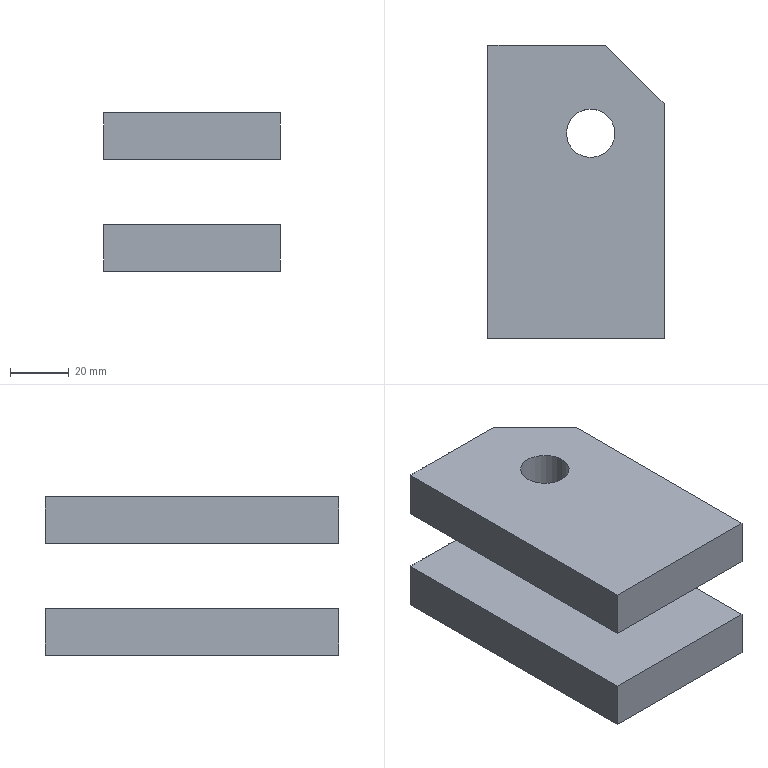Part | SolidWorks | features Chamfer 1, Extrusion 1, ICE 1, MirrorSolid 1 | 2 solids | 18 faces | box 60 x 100 x 54 mm | volume 178758 mm3 | plane 14 | cylinder 4 | commonest cylinder face diameters 16.5 x4
STEP:
#1=CARTESIAN_POINT('',(-3.25,20.,0.));
#2=VERTEX_POINT('',#1);
#3=CARTESIAN_POINT('',(13.25,20.,0.));
#4=VERTEX_POINT('',#3);
#5=CARTESIAN_POINT('',(5.,20.,0.));
#6=DIRECTION('',(0.,0.,1.));
#7=DIRECTION('',(1.,0.,0.));
#8=AXIS2_PLACEMENT_3D('',#5,#6,#7);
#9=CIRCLE('',#8,8.25);
#10=EDGE_CURVE('',#2,#4,#9,.T.);
#11=ORIENTED_EDGE('',*,*,#10,.F.);
#12=CARTESIAN_POINT('',(-3.25,20.,16.));
#13=VERTEX_POINT('',#12);
#14=CARTESIAN_POINT('',(-3.25,20.,0.));
#15=DIRECTION('',(0.,0.,1.));
#16=VECTOR('',#15,1000.);
#17=LINE('',#14,#16);
#18=EDGE_CURVE('',#2,#13,#17,.T.);
#19=ORIENTED_EDGE('',*,*,#18,.T.);
#20=CARTESIAN_POINT('',(13.25,20.,16.));
#21=VERTEX_POINT('',#20);
#22=CARTESIAN_POINT('',(5.,20.,16.));
#23=DIRECTION('',(0.,0.,1.));
#24=DIRECTION('',(1.,0.,0.));
#25=AXIS2_PLACEMENT_3D('',#22,#23,#24);
#26=CIRCLE('',#25,8.25);
#27=EDGE_CURVE('',#13,#21,#26,.T.);
#28=ORIENTED_EDGE('',*,*,#27,.T.);
#29=CARTESIAN_POINT('',(13.25,20.,0.));
#30=DIRECTION('',(0.,0.,1.));
#31=VECTOR('',#30,1000.);
#32=LINE('',#29,#31);
#33=EDGE_CURVE('',#4,#21,#32,.T.);
#34=ORIENTED_EDGE('',*,*,#33,.F.);
#35=EDGE_LOOP('',(#11,#19,#28,#34));
#36=FACE_OUTER_BOUND('',#35,.T.);
#37=CARTESIAN_POINT('',(5.,20.,0.));
#38=DIRECTION('',(0.,0.,1.));
#39=DIRECTION('',(1.,0.,0.));
#40=AXIS2_PLACEMENT_3D('',#37,#38,#39);
#41=CYLINDRICAL_SURFACE('',#40,8.25);
#42=ADVANCED_FACE('',(#36),#41,.F.);
#43=CARTESIAN_POINT('',(30.,-50.,0.));
#44=VERTEX_POINT('',#43);
#45=CARTESIAN_POINT('',(30.,30.,0.));
#46=VERTEX_POINT('',#45);
#47=CARTESIAN_POINT('',(30.,-50.,0.));
#48=DIRECTION('',(0.,1.,0.));
#49=VECTOR('',#48,1000.);
#50=LINE('',#47,#49);
#51=EDGE_CURVE('',#44,#46,#50,.T.);
#52=ORIENTED_EDGE('',*,*,#51,.T.);
#53=CARTESIAN_POINT('',(30.,30.,16.));
#54=VERTEX_POINT('',#53);
#55=CARTESIAN_POINT('',(30.,30.,16.));
#56=DIRECTION('',(0.,0.,1.));
#57=VECTOR('',#56,1000.);
#58=LINE('',#55,#57);
#59=EDGE_CURVE('',#46,#54,#58,.T.);
#60=ORIENTED_EDGE('',*,*,#59,.T.);
#61=CARTESIAN_POINT('',(30.,-50.,16.));
#62=VERTEX_POINT('',#61);
#63=CARTESIAN_POINT('',(30.,-50.,16.));
#64=DIRECTION('',(0.,1.,0.));
#65=VECTOR('',#64,1000.);
#66=LINE('',#63,#65);
#67=EDGE_CURVE('',#62,#54,#66,.T.);
#68=ORIENTED_EDGE('',*,*,#67,.F.);
#69=CARTESIAN_POINT('',(30.,-50.,16.));
#70=DIRECTION('',(0.,0.,-1.));
#71=VECTOR('',#70,1000.);
#72=LINE('',#69,#71);
#73=EDGE_CURVE('',#62,#44,#72,.T.);
#74=ORIENTED_EDGE('',*,*,#73,.T.);
#75=EDGE_LOOP('',(#52,#60,#68,#74));
#76=FACE_OUTER_BOUND('',#75,.T.);
#77=CARTESIAN_POINT('',(30.,-50.,16.));
#78=DIRECTION('',(-1.,0.,0.));
#79=DIRECTION('',(0.,0.,1.));
#80=AXIS2_PLACEMENT_3D('',#77,#78,#79);
#81=PLANE('',#80);
#82=ADVANCED_FACE('',(#76),#81,.F.);
#83=CARTESIAN_POINT('',(10.,50.,16.));
#84=VERTEX_POINT('',#83);
#85=CARTESIAN_POINT('',(-30.,50.,16.));
#86=VERTEX_POINT('',#85);
#87=CARTESIAN_POINT('',(-30.,50.,16.));
#88=DIRECTION('',(-1.,0.,0.));
#89=VECTOR('',#88,1000.);
#90=LINE('',#87,#89);
#91=EDGE_CURVE('',#84,#86,#90,.T.);
#92=ORIENTED_EDGE('',*,*,#91,.F.);
#93=CARTESIAN_POINT('',(10.,50.,0.));
#94=VERTEX_POINT('',#93);
#95=CARTESIAN_POINT('',(10.,50.,16.));
#96=DIRECTION('',(0.,0.,-1.));
#97=VECTOR('',#96,1000.);
#98=LINE('',#95,#97);
#99=EDGE_CURVE('',#84,#94,#98,.T.);
#100=ORIENTED_EDGE('',*,*,#99,.T.);
#101=CARTESIAN_POINT('',(-30.,50.,0.));
#102=VERTEX_POINT('',#101);
#103=CARTESIAN_POINT('',(-30.,50.,0.));
#104=DIRECTION('',(-1.,0.,0.));
#105=VECTOR('',#104,1000.);
#106=LINE('',#103,#105);
#107=EDGE_CURVE('',#94,#102,#106,.T.);
#108=ORIENTED_EDGE('',*,*,#107,.T.);
#109=CARTESIAN_POINT('',(-30.,50.,16.));
#110=DIRECTION('',(0.,0.,-1.));
#111=VECTOR('',#110,1000.);
#112=LINE('',#109,#111);
#113=EDGE_CURVE('',#86,#102,#112,.T.);
#114=ORIENTED_EDGE('',*,*,#113,.F.);
#115=EDGE_LOOP('',(#92,#100,#108,#114));
#116=FACE_OUTER_BOUND('',#115,.T.);
#117=CARTESIAN_POINT('',(-30.,50.,16.));
#118=DIRECTION('',(0.,-1.,0.));
#119=DIRECTION('',(0.,0.,-1.));
#120=AXIS2_PLACEMENT_3D('',#117,#118,#119);
#121=PLANE('',#120);
#122=ADVANCED_FACE('',(#116),#121,.F.);
#123=CARTESIAN_POINT('',(-30.,-50.,0.));
#124=VERTEX_POINT('',#123);
#125=CARTESIAN_POINT('',(-30.,-50.,0.));
#126=DIRECTION('',(0.,-1.,0.));
#127=VECTOR('',#126,1000.);
#128=LINE('',#125,#127);
#129=EDGE_CURVE('',#102,#124,#128,.T.);
#130=ORIENTED_EDGE('',*,*,#129,.T.);
#131=CARTESIAN_POINT('',(-30.,-50.,16.));
#132=VERTEX_POINT('',#131);
#133=CARTESIAN_POINT('',(-30.,-50.,16.));
#134=DIRECTION('',(0.,0.,-1.));
#135=VECTOR('',#134,1000.);
#136=LINE('',#133,#135);
#137=EDGE_CURVE('',#132,#124,#136,.T.);
#138=ORIENTED_EDGE('',*,*,#137,.F.);
#139=CARTESIAN_POINT('',(-30.,-50.,16.));
#140=DIRECTION('',(0.,-1.,0.));
#141=VECTOR('',#140,1000.);
#142=LINE('',#139,#141);
#143=EDGE_CURVE('',#86,#132,#142,.T.);
#144=ORIENTED_EDGE('',*,*,#143,.F.);
#145=ORIENTED_EDGE('',*,*,#113,.T.);
#146=EDGE_LOOP('',(#130,#138,#144,#145));
#147=FACE_OUTER_BOUND('',#146,.T.);
#148=CARTESIAN_POINT('',(-30.,-50.,16.));
#149=DIRECTION('',(1.,0.,0.));
#150=DIRECTION('',(0.,0.,-1.));
#151=AXIS2_PLACEMENT_3D('',#148,#149,#150);
#152=PLANE('',#151);
#153=ADVANCED_FACE('',(#147),#152,.F.);
#154=CARTESIAN_POINT('',(-30.,-50.,0.));
#155=DIRECTION('',(1.,0.,0.));
#156=VECTOR('',#155,1000.);
#157=LINE('',#154,#156);
#158=EDGE_CURVE('',#124,#44,#157,.T.);
#159=ORIENTED_EDGE('',*,*,#158,.T.);
#160=ORIENTED_EDGE('',*,*,#73,.F.);
#161=CARTESIAN_POINT('',(-30.,-50.,16.));
#162=DIRECTION('',(1.,0.,0.));
#163=VECTOR('',#162,1000.);
#164=LINE('',#161,#163);
#165=EDGE_CURVE('',#132,#62,#164,.T.);
#166=ORIENTED_EDGE('',*,*,#165,.F.);
#167=ORIENTED_EDGE('',*,*,#137,.T.);
#168=EDGE_LOOP('',(#159,#160,#166,#167));
#169=FACE_OUTER_BOUND('',#168,.T.);
#170=CARTESIAN_POINT('',(-30.,-50.,16.));
#171=DIRECTION('',(0.,1.,0.));
#172=DIRECTION('',(0.,0.,1.));
#173=AXIS2_PLACEMENT_3D('',#170,#171,#172);
#174=PLANE('',#173);
#175=ADVANCED_FACE('',(#169),#174,.F.);
#176=CARTESIAN_POINT('',(5.,20.,16.));
#177=DIRECTION('',(0.,0.,1.));
#178=DIRECTION('',(1.,0.,0.));
#179=AXIS2_PLACEMENT_3D('',#176,#177,#178);
#180=CIRCLE('',#179,8.25);
#181=EDGE_CURVE('',#21,#13,#180,.T.);
#182=ORIENTED_EDGE('',*,*,#181,.F.);
#183=ORIENTED_EDGE('',*,*,#27,.F.);
#184=EDGE_LOOP('',(#182,#183));
#185=FACE_BOUND('',#184,.T.);
#186=ORIENTED_EDGE('',*,*,#67,.T.);
#187=CARTESIAN_POINT('',(10.,50.,16.));
#188=DIRECTION('',(-0.7071,0.7071,0.));
#189=VECTOR('',#188,1000.);
#190=LINE('',#187,#189);
#191=EDGE_CURVE('',#54,#84,#190,.T.);
#192=ORIENTED_EDGE('',*,*,#191,.T.);
#193=ORIENTED_EDGE('',*,*,#91,.T.);
#194=ORIENTED_EDGE('',*,*,#143,.T.);
#195=ORIENTED_EDGE('',*,*,#165,.T.);
#196=EDGE_LOOP('',(#186,#192,#193,#194,#195));
#197=FACE_OUTER_BOUND('',#196,.T.);
#198=CARTESIAN_POINT('',(0.,0.,16.));
#199=DIRECTION('',(0.,0.,-1.));
#200=DIRECTION('',(-1.,0.,0.));
#201=AXIS2_PLACEMENT_3D('',#198,#199,#200);
#202=PLANE('',#201);
#203=ADVANCED_FACE('',(#185,#197),#202,.F.);
#204=CARTESIAN_POINT('',(5.,20.,0.));
#205=DIRECTION('',(0.,0.,1.));
#206=DIRECTION('',(1.,0.,0.));
#207=AXIS2_PLACEMENT_3D('',#204,#205,#206);
#208=CIRCLE('',#207,8.25);
#209=EDGE_CURVE('',#4,#2,#208,.T.);
#210=ORIENTED_EDGE('',*,*,#209,.T.);
#211=ORIENTED_EDGE('',*,*,#10,.T.);
#212=EDGE_LOOP('',(#210,#211));
#213=FACE_BOUND('',#212,.T.);
#214=ORIENTED_EDGE('',*,*,#107,.F.);
#215=CARTESIAN_POINT('',(30.,30.,0.));
#216=DIRECTION('',(0.7071,-0.7071,0.));
#217=VECTOR('',#216,1000.);
#218=LINE('',#215,#217);
#219=EDGE_CURVE('',#94,#46,#218,.T.);
#220=ORIENTED_EDGE('',*,*,#219,.T.);
#221=ORIENTED_EDGE('',*,*,#51,.F.);
#222=ORIENTED_EDGE('',*,*,#158,.F.);
#223=ORIENTED_EDGE('',*,*,#129,.F.);
#224=EDGE_LOOP('',(#214,#220,#221,#222,#223));
#225=FACE_OUTER_BOUND('',#224,.T.);
#226=CARTESIAN_POINT('',(0.,0.,0.));
#227=DIRECTION('',(0.,0.,-1.));
#228=DIRECTION('',(-1.,0.,0.));
#229=AXIS2_PLACEMENT_3D('',#226,#227,#228);
#230=PLANE('',#229);
#231=ADVANCED_FACE('',(#213,#225),#230,.T.);
#232=ORIENTED_EDGE('',*,*,#18,.F.);
#233=ORIENTED_EDGE('',*,*,#209,.F.);
#234=ORIENTED_EDGE('',*,*,#33,.T.);
#235=ORIENTED_EDGE('',*,*,#181,.T.);
#236=EDGE_LOOP('',(#232,#233,#234,#235));
#237=FACE_OUTER_BOUND('',#236,.T.);
#238=CARTESIAN_POINT('',(5.,20.,0.));
#239=DIRECTION('',(0.,0.,1.));
#240=DIRECTION('',(1.,0.,0.));
#241=AXIS2_PLACEMENT_3D('',#238,#239,#240);
#242=CYLINDRICAL_SURFACE('',#241,8.25);
#243=ADVANCED_FACE('',(#237),#242,.F.);
#244=ORIENTED_EDGE('',*,*,#191,.F.);
#245=ORIENTED_EDGE('',*,*,#59,.F.);
#246=ORIENTED_EDGE('',*,*,#219,.F.);
#247=ORIENTED_EDGE('',*,*,#99,.F.);
#248=EDGE_LOOP('',(#244,#245,#246,#247));
#249=FACE_OUTER_BOUND('',#248,.T.);
#250=CARTESIAN_POINT('',(10.,50.,16.));
#251=DIRECTION('',(-0.7071,-0.7071,0.));
#252=DIRECTION('',(0.,0.,-1.));
#253=AXIS2_PLACEMENT_3D('',#250,#251,#252);
#254=PLANE('',#253);
#255=ADVANCED_FACE('',(#249),#254,.F.);
#256=CLOSED_SHELL('',(#42,#82,#122,#153,#175,#203,#231,#243,#255));
#257=MANIFOLD_SOLID_BREP('',#256);
#258=CARTESIAN_POINT('',(13.25,20.,-22.));
#259=VERTEX_POINT('',#258);
#260=CARTESIAN_POINT('',(-3.25,20.,-22.));
#261=VERTEX_POINT('',#260);
#262=CARTESIAN_POINT('',(5.,20.,-22.));
#263=DIRECTION('',(0.,0.,1.));
#264=DIRECTION('',(1.,0.,0.));
#265=AXIS2_PLACEMENT_3D('',#262,#263,#264);
#266=CIRCLE('',#265,8.25);
#267=EDGE_CURVE('',#259,#261,#266,.T.);
#268=ORIENTED_EDGE('',*,*,#267,.T.);
#269=CARTESIAN_POINT('',(-3.25,20.,-38.));
#270=VERTEX_POINT('',#269);
#271=CARTESIAN_POINT('',(-3.25,20.,-22.));
#272=DIRECTION('',(0.,0.,-1.));
#273=VECTOR('',#272,1000.);
#274=LINE('',#271,#273);
#275=EDGE_CURVE('',#261,#270,#274,.T.);
#276=ORIENTED_EDGE('',*,*,#275,.T.);
#277=CARTESIAN_POINT('',(13.25,20.,-38.));
#278=VERTEX_POINT('',#277);
#279=CARTESIAN_POINT('',(5.,20.,-38.));
#280=DIRECTION('',(0.,0.,1.));
#281=DIRECTION('',(1.,0.,0.));
#282=AXIS2_PLACEMENT_3D('',#279,#280,#281);
#283=CIRCLE('',#282,8.25);
#284=EDGE_CURVE('',#278,#270,#283,.T.);
#285=ORIENTED_EDGE('',*,*,#284,.F.);
#286=CARTESIAN_POINT('',(13.25,20.,-22.));
#287=DIRECTION('',(0.,0.,-1.));
#288=VECTOR('',#287,1000.);
#289=LINE('',#286,#288);
#290=EDGE_CURVE('',#259,#278,#289,.T.);
#291=ORIENTED_EDGE('',*,*,#290,.F.);
#292=EDGE_LOOP('',(#268,#276,#285,#291));
#293=FACE_OUTER_BOUND('',#292,.T.);
#294=CARTESIAN_POINT('',(5.,20.,-22.));
#295=DIRECTION('',(0.,0.,-1.));
#296=DIRECTION('',(1.,0.,0.));
#297=AXIS2_PLACEMENT_3D('',#294,#295,#296);
#298=CYLINDRICAL_SURFACE('',#297,8.25);
#299=ADVANCED_FACE('',(#293),#298,.F.);
#300=CARTESIAN_POINT('',(30.,-50.,-22.));
#301=VERTEX_POINT('',#300);
#302=CARTESIAN_POINT('',(30.,30.,-22.));
#303=VERTEX_POINT('',#302);
#304=CARTESIAN_POINT('',(30.,-50.,-22.));
#305=DIRECTION('',(0.,1.,0.));
#306=VECTOR('',#305,1000.);
#307=LINE('',#304,#306);
#308=EDGE_CURVE('',#301,#303,#307,.T.);
#309=ORIENTED_EDGE('',*,*,#308,.F.);
#310=CARTESIAN_POINT('',(30.,-50.,-38.));
#311=VERTEX_POINT('',#310);
#312=CARTESIAN_POINT('',(30.,-50.,-38.));
#313=DIRECTION('',(0.,0.,1.));
#314=VECTOR('',#313,1000.);
#315=LINE('',#312,#314);
#316=EDGE_CURVE('',#311,#301,#315,.T.);
#317=ORIENTED_EDGE('',*,*,#316,.F.);
#318=CARTESIAN_POINT('',(30.,30.,-38.));
#319=VERTEX_POINT('',#318);
#320=CARTESIAN_POINT('',(30.,-50.,-38.));
#321=DIRECTION('',(0.,1.,0.));
#322=VECTOR('',#321,1000.);
#323=LINE('',#320,#322);
#324=EDGE_CURVE('',#311,#319,#323,.T.);
#325=ORIENTED_EDGE('',*,*,#324,.T.);
#326=CARTESIAN_POINT('',(30.,30.,-38.));
#327=DIRECTION('',(0.,0.,-1.));
#328=VECTOR('',#327,1000.);
#329=LINE('',#326,#328);
#330=EDGE_CURVE('',#303,#319,#329,.T.);
#331=ORIENTED_EDGE('',*,*,#330,.F.);
#332=EDGE_LOOP('',(#309,#317,#325,#331));
#333=FACE_OUTER_BOUND('',#332,.T.);
#334=CARTESIAN_POINT('',(30.,-50.,-38.));
#335=DIRECTION('',(-1.,0.,0.));
#336=DIRECTION('',(0.,0.,-1.));
#337=AXIS2_PLACEMENT_3D('',#334,#335,#336);
#338=PLANE('',#337);
#339=ADVANCED_FACE('',(#333),#338,.F.);
#340=CARTESIAN_POINT('',(10.,50.,-38.));
#341=VERTEX_POINT('',#340);
#342=CARTESIAN_POINT('',(-30.,50.,-38.));
#343=VERTEX_POINT('',#342);
#344=CARTESIAN_POINT('',(-30.,50.,-38.));
#345=DIRECTION('',(-1.,0.,0.));
#346=VECTOR('',#345,1000.);
#347=LINE('',#344,#346);
#348=EDGE_CURVE('',#341,#343,#347,.T.);
#349=ORIENTED_EDGE('',*,*,#348,.T.);
#350=CARTESIAN_POINT('',(-30.,50.,-22.));
#351=VERTEX_POINT('',#350);
#352=CARTESIAN_POINT('',(-30.,50.,-38.));
#353=DIRECTION('',(0.,0.,1.));
#354=VECTOR('',#353,1000.);
#355=LINE('',#352,#354);
#356=EDGE_CURVE('',#343,#351,#355,.T.);
#357=ORIENTED_EDGE('',*,*,#356,.T.);
#358=CARTESIAN_POINT('',(10.,50.,-22.));
#359=VERTEX_POINT('',#358);
#360=CARTESIAN_POINT('',(-30.,50.,-22.));
#361=DIRECTION('',(-1.,0.,0.));
#362=VECTOR('',#361,1000.);
#363=LINE('',#360,#362);
#364=EDGE_CURVE('',#359,#351,#363,.T.);
#365=ORIENTED_EDGE('',*,*,#364,.F.);
#366=CARTESIAN_POINT('',(10.,50.,-38.));
#367=DIRECTION('',(0.,0.,1.));
#368=VECTOR('',#367,1000.);
#369=LINE('',#366,#368);
#370=EDGE_CURVE('',#341,#359,#369,.T.);
#371=ORIENTED_EDGE('',*,*,#370,.F.);
#372=EDGE_LOOP('',(#349,#357,#365,#371));
#373=FACE_OUTER_BOUND('',#372,.T.);
#374=CARTESIAN_POINT('',(-30.,50.,-38.));
#375=DIRECTION('',(0.,-1.,0.));
#376=DIRECTION('',(0.,0.,1.));
#377=AXIS2_PLACEMENT_3D('',#374,#375,#376);
#378=PLANE('',#377);
#379=ADVANCED_FACE('',(#373),#378,.F.);
#380=CARTESIAN_POINT('',(-30.,-50.,-22.));
#381=VERTEX_POINT('',#380);
#382=CARTESIAN_POINT('',(-30.,-50.,-22.));
#383=DIRECTION('',(0.,-1.,0.));
#384=VECTOR('',#383,1000.);
#385=LINE('',#382,#384);
#386=EDGE_CURVE('',#351,#381,#385,.T.);
#387=ORIENTED_EDGE('',*,*,#386,.F.);
#388=ORIENTED_EDGE('',*,*,#356,.F.);
#389=CARTESIAN_POINT('',(-30.,-50.,-38.));
#390=VERTEX_POINT('',#389);
#391=CARTESIAN_POINT('',(-30.,-50.,-38.));
#392=DIRECTION('',(0.,-1.,0.));
#393=VECTOR('',#392,1000.);
#394=LINE('',#391,#393);
#395=EDGE_CURVE('',#343,#390,#394,.T.);
#396=ORIENTED_EDGE('',*,*,#395,.T.);
#397=CARTESIAN_POINT('',(-30.,-50.,-38.));
#398=DIRECTION('',(0.,0.,1.));
#399=VECTOR('',#398,1000.);
#400=LINE('',#397,#399);
#401=EDGE_CURVE('',#390,#381,#400,.T.);
#402=ORIENTED_EDGE('',*,*,#401,.T.);
#403=EDGE_LOOP('',(#387,#388,#396,#402));
#404=FACE_OUTER_BOUND('',#403,.T.);
#405=CARTESIAN_POINT('',(-30.,-50.,-38.));
#406=DIRECTION('',(1.,0.,0.));
#407=DIRECTION('',(0.,0.,1.));
#408=AXIS2_PLACEMENT_3D('',#405,#406,#407);
#409=PLANE('',#408);
#410=ADVANCED_FACE('',(#404),#409,.F.);
#411=CARTESIAN_POINT('',(-30.,-50.,-22.));
#412=DIRECTION('',(1.,0.,0.));
#413=VECTOR('',#412,1000.);
#414=LINE('',#411,#413);
#415=EDGE_CURVE('',#381,#301,#414,.T.);
#416=ORIENTED_EDGE('',*,*,#415,.F.);
#417=ORIENTED_EDGE('',*,*,#401,.F.);
#418=CARTESIAN_POINT('',(-30.,-50.,-38.));
#419=DIRECTION('',(1.,0.,0.));
#420=VECTOR('',#419,1000.);
#421=LINE('',#418,#420);
#422=EDGE_CURVE('',#390,#311,#421,.T.);
#423=ORIENTED_EDGE('',*,*,#422,.T.);
#424=ORIENTED_EDGE('',*,*,#316,.T.);
#425=EDGE_LOOP('',(#416,#417,#423,#424));
#426=FACE_OUTER_BOUND('',#425,.T.);
#427=CARTESIAN_POINT('',(-30.,-50.,-38.));
#428=DIRECTION('',(0.,1.,0.));
#429=DIRECTION('',(0.,0.,-1.));
#430=AXIS2_PLACEMENT_3D('',#427,#428,#429);
#431=PLANE('',#430);
#432=ADVANCED_FACE('',(#426),#431,.F.);
#433=ORIENTED_EDGE('',*,*,#284,.T.);
#434=CARTESIAN_POINT('',(5.,20.,-38.));
#435=DIRECTION('',(0.,0.,1.));
#436=DIRECTION('',(1.,0.,0.));
#437=AXIS2_PLACEMENT_3D('',#434,#435,#436);
#438=CIRCLE('',#437,8.25);
#439=EDGE_CURVE('',#270,#278,#438,.T.);
#440=ORIENTED_EDGE('',*,*,#439,.T.);
#441=EDGE_LOOP('',(#433,#440));
#442=FACE_BOUND('',#441,.T.);
#443=ORIENTED_EDGE('',*,*,#324,.F.);
#444=ORIENTED_EDGE('',*,*,#422,.F.);
#445=ORIENTED_EDGE('',*,*,#395,.F.);
#446=ORIENTED_EDGE('',*,*,#348,.F.);
#447=CARTESIAN_POINT('',(10.,50.,-38.));
#448=DIRECTION('',(-0.7071,0.7071,0.));
#449=VECTOR('',#448,1000.);
#450=LINE('',#447,#449);
#451=EDGE_CURVE('',#319,#341,#450,.T.);
#452=ORIENTED_EDGE('',*,*,#451,.F.);
#453=EDGE_LOOP('',(#443,#444,#445,#446,#452));
#454=FACE_OUTER_BOUND('',#453,.T.);
#455=CARTESIAN_POINT('',(0.,0.,-38.));
#456=DIRECTION('',(0.,0.,1.));
#457=DIRECTION('',(-1.,0.,0.));
#458=AXIS2_PLACEMENT_3D('',#455,#456,#457);
#459=PLANE('',#458);
#460=ADVANCED_FACE('',(#442,#454),#459,.F.);
#461=ORIENTED_EDGE('',*,*,#267,.F.);
#462=CARTESIAN_POINT('',(5.,20.,-22.));
#463=DIRECTION('',(0.,0.,1.));
#464=DIRECTION('',(1.,0.,0.));
#465=AXIS2_PLACEMENT_3D('',#462,#463,#464);
#466=CIRCLE('',#465,8.25);
#467=EDGE_CURVE('',#261,#259,#466,.T.);
#468=ORIENTED_EDGE('',*,*,#467,.F.);
#469=EDGE_LOOP('',(#461,#468));
#470=FACE_BOUND('',#469,.T.);
#471=ORIENTED_EDGE('',*,*,#364,.T.);
#472=ORIENTED_EDGE('',*,*,#386,.T.);
#473=ORIENTED_EDGE('',*,*,#415,.T.);
#474=ORIENTED_EDGE('',*,*,#308,.T.);
#475=CARTESIAN_POINT('',(30.,30.,-22.));
#476=DIRECTION('',(0.7071,-0.7071,0.));
#477=VECTOR('',#476,1000.);
#478=LINE('',#475,#477);
#479=EDGE_CURVE('',#359,#303,#478,.T.);
#480=ORIENTED_EDGE('',*,*,#479,.F.);
#481=EDGE_LOOP('',(#471,#472,#473,#474,#480));
#482=FACE_OUTER_BOUND('',#481,.T.);
#483=CARTESIAN_POINT('',(0.,0.,-22.));
#484=DIRECTION('',(0.,0.,1.));
#485=DIRECTION('',(-1.,0.,0.));
#486=AXIS2_PLACEMENT_3D('',#483,#484,#485);
#487=PLANE('',#486);
#488=ADVANCED_FACE('',(#470,#482),#487,.T.);
#489=ORIENTED_EDGE('',*,*,#275,.F.);
#490=ORIENTED_EDGE('',*,*,#467,.T.);
#491=ORIENTED_EDGE('',*,*,#290,.T.);
#492=ORIENTED_EDGE('',*,*,#439,.F.);
#493=EDGE_LOOP('',(#489,#490,#491,#492));
#494=FACE_OUTER_BOUND('',#493,.T.);
#495=CARTESIAN_POINT('',(5.,20.,-22.));
#496=DIRECTION('',(0.,0.,-1.));
#497=DIRECTION('',(1.,0.,0.));
#498=AXIS2_PLACEMENT_3D('',#495,#496,#497);
#499=CYLINDRICAL_SURFACE('',#498,8.25);
#500=ADVANCED_FACE('',(#494),#499,.F.);
#501=ORIENTED_EDGE('',*,*,#451,.T.);
#502=ORIENTED_EDGE('',*,*,#370,.T.);
#503=ORIENTED_EDGE('',*,*,#479,.T.);
#504=ORIENTED_EDGE('',*,*,#330,.T.);
#505=EDGE_LOOP('',(#501,#502,#503,#504));
#506=FACE_OUTER_BOUND('',#505,.T.);
#507=CARTESIAN_POINT('',(10.,50.,-38.));
#508=DIRECTION('',(-0.7071,-0.7071,0.));
#509=DIRECTION('',(0.,0.,1.));
#510=AXIS2_PLACEMENT_3D('',#507,#508,#509);
#511=PLANE('',#510);
#512=ADVANCED_FACE('',(#506),#511,.F.);
#513=CLOSED_SHELL('',(#299,#339,#379,#410,#432,#460,#488,#500,#512));
#514=MANIFOLD_SOLID_BREP('',#513);
#515=CARTESIAN_POINT('',(0.,0.,0.));
#516=DIRECTION('',(0.,0.,1.));
#517=DIRECTION('',(1.,0.,0.));
#518=AXIS2_PLACEMENT_3D('',#515,#516,#517);
#519=(LENGTH_UNIT()NAMED_UNIT(*)SI_UNIT(.MILLI.,.METRE.));
#520=UNCERTAINTY_MEASURE_WITH_UNIT(LENGTH_MEASURE(0.00001),#519,'','');
#521=(NAMED_UNIT(*)PLANE_ANGLE_UNIT()SI_UNIT($,.RADIAN.));
#522=(NAMED_UNIT(*)SI_UNIT($,.STERADIAN.)SOLID_ANGLE_UNIT());
#523=(GEOMETRIC_REPRESENTATION_CONTEXT(3)GLOBAL_UNCERTAINTY_ASSIGNED_CONTEXT((#520))GLOBAL_UNIT_ASSIGNED_CONTEXT((#519,#521,#522))REPRESENTATION_CONTEXT('',''));
#524=ADVANCED_BREP_SHAPE_REPRESENTATION('',(#257,#514,#518),#523);